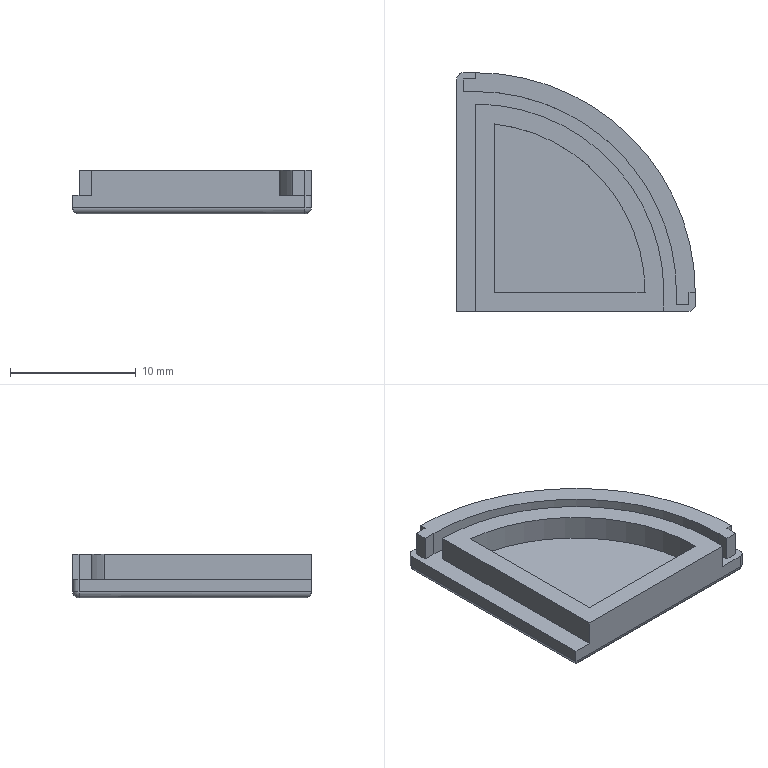Part | SolidWorks | features Extrusion 1, Fillet 1, ICE 1 | 1 solid | 34 faces | box 19 x 19 x 3.5 mm | volume 674.646 mm3 | plane 21 | cylinder 10 | sphere 2 | torus 1 | commonest cylinder face diameters 1 x6 27 x1 30 x1 32 x1 35 x1
STEP:
#1=CARTESIAN_POINT('',(16.5,0.,1.5));
#2=VERTEX_POINT('',#1);
#3=CARTESIAN_POINT('',(18.5,0.,1.5));
#4=VERTEX_POINT('',#3);
#5=CARTESIAN_POINT('',(19.,0.,1.5));
#6=DIRECTION('',(1.,0.,0.));
#7=VECTOR('',#6,1000.);
#8=LINE('',#5,#7);
#9=EDGE_CURVE('',#2,#4,#8,.T.);
#10=ORIENTED_EDGE('',*,*,#9,.T.);
#11=CARTESIAN_POINT('',(19.,0.5,1.5));
#12=VERTEX_POINT('',#11);
#13=CARTESIAN_POINT('',(18.5,0.5,1.5));
#14=DIRECTION('',(0.,0.,1.));
#15=DIRECTION('',(-1.,0.,0.));
#16=AXIS2_PLACEMENT_3D('',#13,#14,#15);
#17=CIRCLE('',#16,0.5);
#18=EDGE_CURVE('',#4,#12,#17,.T.);
#19=ORIENTED_EDGE('',*,*,#18,.T.);
#20=CARTESIAN_POINT('',(19.,1.5,1.5));
#21=VERTEX_POINT('',#20);
#22=CARTESIAN_POINT('',(19.,1.5,1.5));
#23=DIRECTION('',(0.,1.,0.));
#24=VECTOR('',#23,1000.);
#25=LINE('',#22,#24);
#26=EDGE_CURVE('',#12,#21,#25,.T.);
#27=ORIENTED_EDGE('',*,*,#26,.T.);
#28=CARTESIAN_POINT('',(18.5,1.5,1.5));
#29=VERTEX_POINT('',#28);
#30=CARTESIAN_POINT('',(18.5,1.5,1.5));
#31=DIRECTION('',(1.,0.,0.));
#32=VECTOR('',#31,1000.);
#33=LINE('',#30,#32);
#34=EDGE_CURVE('',#29,#21,#33,.T.);
#35=ORIENTED_EDGE('',*,*,#34,.F.);
#36=CARTESIAN_POINT('',(18.5,0.5,1.5));
#37=VERTEX_POINT('',#36);
#38=CARTESIAN_POINT('',(18.5,0.5,1.5));
#39=DIRECTION('',(0.,1.,0.));
#40=VECTOR('',#39,1000.);
#41=LINE('',#38,#40);
#42=EDGE_CURVE('',#37,#29,#41,.T.);
#43=ORIENTED_EDGE('',*,*,#42,.F.);
#44=CARTESIAN_POINT('',(17.5,0.5,1.5));
#45=VERTEX_POINT('',#44);
#46=CARTESIAN_POINT('',(17.5,0.5,1.5));
#47=DIRECTION('',(1.,0.,0.));
#48=VECTOR('',#47,1000.);
#49=LINE('',#46,#48);
#50=EDGE_CURVE('',#45,#37,#49,.T.);
#51=ORIENTED_EDGE('',*,*,#50,.F.);
#52=CARTESIAN_POINT('',(17.5,1.5,1.5));
#53=VERTEX_POINT('',#52);
#54=CARTESIAN_POINT('',(17.5,1.5,1.5));
#55=DIRECTION('',(0.,-1.,0.));
#56=VECTOR('',#55,1000.);
#57=LINE('',#54,#56);
#58=EDGE_CURVE('',#53,#45,#57,.T.);
#59=ORIENTED_EDGE('',*,*,#58,.F.);
#60=CARTESIAN_POINT('',(1.5,17.5,1.5));
#61=VERTEX_POINT('',#60);
#62=CARTESIAN_POINT('',(1.5,1.5,1.5));
#63=DIRECTION('',(0.,0.,-1.));
#64=DIRECTION('',(-1.,0.,0.));
#65=AXIS2_PLACEMENT_3D('',#62,#63,#64);
#66=CIRCLE('',#65,16.);
#67=EDGE_CURVE('',#61,#53,#66,.T.);
#68=ORIENTED_EDGE('',*,*,#67,.F.);
#69=CARTESIAN_POINT('',(0.5,17.5,1.5));
#70=VERTEX_POINT('',#69);
#71=CARTESIAN_POINT('',(0.5,17.5,1.5));
#72=DIRECTION('',(1.,0.,0.));
#73=VECTOR('',#72,1000.);
#74=LINE('',#71,#73);
#75=EDGE_CURVE('',#70,#61,#74,.T.);
#76=ORIENTED_EDGE('',*,*,#75,.F.);
#77=CARTESIAN_POINT('',(0.5,18.5,1.5));
#78=VERTEX_POINT('',#77);
#79=CARTESIAN_POINT('',(0.5,18.5,1.5));
#80=DIRECTION('',(0.,-1.,0.));
#81=VECTOR('',#80,1000.);
#82=LINE('',#79,#81);
#83=EDGE_CURVE('',#78,#70,#82,.T.);
#84=ORIENTED_EDGE('',*,*,#83,.F.);
#85=CARTESIAN_POINT('',(1.5,18.5,1.5));
#86=VERTEX_POINT('',#85);
#87=CARTESIAN_POINT('',(1.5,18.5,1.5));
#88=DIRECTION('',(-1.,0.,0.));
#89=VECTOR('',#88,1000.);
#90=LINE('',#87,#89);
#91=EDGE_CURVE('',#86,#78,#90,.T.);
#92=ORIENTED_EDGE('',*,*,#91,.F.);
#93=CARTESIAN_POINT('',(1.5,19.,1.5));
#94=VERTEX_POINT('',#93);
#95=CARTESIAN_POINT('',(1.5,19.,1.5));
#96=DIRECTION('',(0.,-1.,0.));
#97=VECTOR('',#96,1000.);
#98=LINE('',#95,#97);
#99=EDGE_CURVE('',#94,#86,#98,.T.);
#100=ORIENTED_EDGE('',*,*,#99,.F.);
#101=CARTESIAN_POINT('',(0.5,19.,1.5));
#102=VERTEX_POINT('',#101);
#103=CARTESIAN_POINT('',(0.,19.,1.5));
#104=DIRECTION('',(-1.,0.,0.));
#105=VECTOR('',#104,1000.);
#106=LINE('',#103,#105);
#107=EDGE_CURVE('',#94,#102,#106,.T.);
#108=ORIENTED_EDGE('',*,*,#107,.T.);
#109=CARTESIAN_POINT('',(0.,18.5,1.5));
#110=VERTEX_POINT('',#109);
#111=CARTESIAN_POINT('',(0.5,18.5,1.5));
#112=DIRECTION('',(0.,0.,1.));
#113=DIRECTION('',(-1.,0.,0.));
#114=AXIS2_PLACEMENT_3D('',#111,#112,#113);
#115=CIRCLE('',#114,0.5);
#116=EDGE_CURVE('',#102,#110,#115,.T.);
#117=ORIENTED_EDGE('',*,*,#116,.T.);
#118=CARTESIAN_POINT('',(0.,0.,1.5));
#119=VERTEX_POINT('',#118);
#120=CARTESIAN_POINT('',(0.,0.,1.5));
#121=DIRECTION('',(0.,-1.,0.));
#122=VECTOR('',#121,1000.);
#123=LINE('',#120,#122);
#124=EDGE_CURVE('',#110,#119,#123,.T.);
#125=ORIENTED_EDGE('',*,*,#124,.T.);
#126=CARTESIAN_POINT('',(1.5,0.,1.5));
#127=VERTEX_POINT('',#126);
#128=CARTESIAN_POINT('',(19.,0.,1.5));
#129=DIRECTION('',(1.,0.,0.));
#130=VECTOR('',#129,1000.);
#131=LINE('',#128,#130);
#132=EDGE_CURVE('',#119,#127,#131,.T.);
#133=ORIENTED_EDGE('',*,*,#132,.T.);
#134=CARTESIAN_POINT('',(1.5,16.5,1.5));
#135=VERTEX_POINT('',#134);
#136=CARTESIAN_POINT('',(1.5,16.5,1.5));
#137=DIRECTION('',(0.,-1.,0.));
#138=VECTOR('',#137,1000.);
#139=LINE('',#136,#138);
#140=EDGE_CURVE('',#135,#127,#139,.T.);
#141=ORIENTED_EDGE('',*,*,#140,.F.);
#142=CARTESIAN_POINT('',(16.5,1.5,1.5));
#143=VERTEX_POINT('',#142);
#144=CARTESIAN_POINT('',(1.5,1.5,1.5));
#145=DIRECTION('',(0.,0.,1.));
#146=DIRECTION('',(1.,0.,0.));
#147=AXIS2_PLACEMENT_3D('',#144,#145,#146);
#148=CIRCLE('',#147,15.);
#149=EDGE_CURVE('',#143,#135,#148,.T.);
#150=ORIENTED_EDGE('',*,*,#149,.F.);
#151=CARTESIAN_POINT('',(16.5,0.,1.5));
#152=DIRECTION('',(0.,1.,0.));
#153=VECTOR('',#152,1000.);
#154=LINE('',#151,#153);
#155=EDGE_CURVE('',#2,#143,#154,.T.);
#156=ORIENTED_EDGE('',*,*,#155,.F.);
#157=EDGE_LOOP('',(#10,#19,#27,#35,#43,#51,#59,#68,#76,#84,#92,#100,#108,#117,#125,#133,#141,#150,#156));
#158=FACE_OUTER_BOUND('',#157,.T.);
#159=CARTESIAN_POINT('',(1.5,1.5,1.5));
#160=DIRECTION('',(0.,0.,-1.));
#161=DIRECTION('',(-1.,0.,0.));
#162=AXIS2_PLACEMENT_3D('',#159,#160,#161);
#163=PLANE('',#162);
#164=ADVANCED_FACE('',(#158),#163,.F.);
#165=CARTESIAN_POINT('',(0.,0.,0.5));
#166=VERTEX_POINT('',#165);
#167=CARTESIAN_POINT('',(18.5,0.,0.5));
#168=VERTEX_POINT('',#167);
#169=CARTESIAN_POINT('',(19.,0.,0.5));
#170=DIRECTION('',(1.,0.,0.));
#171=VECTOR('',#170,1000.);
#172=LINE('',#169,#171);
#173=EDGE_CURVE('',#166,#168,#172,.T.);
#174=ORIENTED_EDGE('',*,*,#173,.T.);
#175=CARTESIAN_POINT('',(18.5,0.,1.5));
#176=DIRECTION('',(0.,0.,1.));
#177=VECTOR('',#176,1000.);
#178=LINE('',#175,#177);
#179=EDGE_CURVE('',#168,#4,#178,.T.);
#180=ORIENTED_EDGE('',*,*,#179,.T.);
#181=ORIENTED_EDGE('',*,*,#9,.F.);
#182=CARTESIAN_POINT('',(16.5,0.,3.5));
#183=VERTEX_POINT('',#182);
#184=CARTESIAN_POINT('',(16.5,0.,3.5));
#185=DIRECTION('',(0.,0.,-1.));
#186=VECTOR('',#185,1000.);
#187=LINE('',#184,#186);
#188=EDGE_CURVE('',#183,#2,#187,.T.);
#189=ORIENTED_EDGE('',*,*,#188,.F.);
#190=CARTESIAN_POINT('',(1.5,0.,3.5));
#191=VERTEX_POINT('',#190);
#192=CARTESIAN_POINT('',(1.5,0.,3.5));
#193=DIRECTION('',(1.,0.,0.));
#194=VECTOR('',#193,1000.);
#195=LINE('',#192,#194);
#196=EDGE_CURVE('',#191,#183,#195,.T.);
#197=ORIENTED_EDGE('',*,*,#196,.F.);
#198=CARTESIAN_POINT('',(1.5,0.,3.5));
#199=DIRECTION('',(0.,0.,-1.));
#200=VECTOR('',#199,1000.);
#201=LINE('',#198,#200);
#202=EDGE_CURVE('',#191,#127,#201,.T.);
#203=ORIENTED_EDGE('',*,*,#202,.T.);
#204=ORIENTED_EDGE('',*,*,#132,.F.);
#205=CARTESIAN_POINT('',(0.,0.,1.5));
#206=DIRECTION('',(0.,0.,-1.));
#207=VECTOR('',#206,1000.);
#208=LINE('',#205,#207);
#209=EDGE_CURVE('',#119,#166,#208,.T.);
#210=ORIENTED_EDGE('',*,*,#209,.T.);
#211=EDGE_LOOP('',(#174,#180,#181,#189,#197,#203,#204,#210));
#212=FACE_OUTER_BOUND('',#211,.T.);
#213=CARTESIAN_POINT('',(19.,0.,1.5));
#214=DIRECTION('',(0.,1.,0.));
#215=DIRECTION('',(0.,0.,1.));
#216=AXIS2_PLACEMENT_3D('',#213,#214,#215);
#217=PLANE('',#216);
#218=ADVANCED_FACE('',(#212),#217,.F.);
#219=CARTESIAN_POINT('',(19.,0.5,0.5));
#220=VERTEX_POINT('',#219);
#221=CARTESIAN_POINT('',(19.,0.5,1.5));
#222=DIRECTION('',(0.,0.,-1.));
#223=VECTOR('',#222,1000.);
#224=LINE('',#221,#223);
#225=EDGE_CURVE('',#12,#220,#224,.T.);
#226=ORIENTED_EDGE('',*,*,#225,.T.);
#227=CARTESIAN_POINT('',(19.,1.5,0.5));
#228=VERTEX_POINT('',#227);
#229=CARTESIAN_POINT('',(19.,1.5,0.5));
#230=DIRECTION('',(0.,1.,0.));
#231=VECTOR('',#230,1000.);
#232=LINE('',#229,#231);
#233=EDGE_CURVE('',#220,#228,#232,.T.);
#234=ORIENTED_EDGE('',*,*,#233,.T.);
#235=CARTESIAN_POINT('',(19.,1.5,1.5));
#236=DIRECTION('',(0.,0.,-1.));
#237=VECTOR('',#236,1000.);
#238=LINE('',#235,#237);
#239=EDGE_CURVE('',#21,#228,#238,.T.);
#240=ORIENTED_EDGE('',*,*,#239,.F.);
#241=ORIENTED_EDGE('',*,*,#26,.F.);
#242=EDGE_LOOP('',(#226,#234,#240,#241));
#243=FACE_OUTER_BOUND('',#242,.T.);
#244=CARTESIAN_POINT('',(19.,1.5,1.5));
#245=DIRECTION('',(-1.,0.,0.));
#246=DIRECTION('',(0.,0.,1.));
#247=AXIS2_PLACEMENT_3D('',#244,#245,#246);
#248=PLANE('',#247);
#249=ADVANCED_FACE('',(#243),#248,.F.);
#250=ORIENTED_EDGE('',*,*,#239,.T.);
#251=CARTESIAN_POINT('',(1.5,19.,0.5));
#252=VERTEX_POINT('',#251);
#253=CARTESIAN_POINT('',(1.5,1.5,0.5));
#254=DIRECTION('',(0.,0.,1.));
#255=DIRECTION('',(-1.,0.,0.));
#256=AXIS2_PLACEMENT_3D('',#253,#254,#255);
#257=CIRCLE('',#256,17.5);
#258=EDGE_CURVE('',#228,#252,#257,.T.);
#259=ORIENTED_EDGE('',*,*,#258,.T.);
#260=CARTESIAN_POINT('',(1.5,19.,1.5));
#261=DIRECTION('',(0.,0.,-1.));
#262=VECTOR('',#261,1000.);
#263=LINE('',#260,#262);
#264=EDGE_CURVE('',#94,#252,#263,.T.);
#265=ORIENTED_EDGE('',*,*,#264,.F.);
#266=CARTESIAN_POINT('',(1.5,19.,3.5));
#267=VERTEX_POINT('',#266);
#268=CARTESIAN_POINT('',(1.5,19.,3.5));
#269=DIRECTION('',(0.,0.,-1.));
#270=VECTOR('',#269,1000.);
#271=LINE('',#268,#270);
#272=EDGE_CURVE('',#267,#94,#271,.T.);
#273=ORIENTED_EDGE('',*,*,#272,.F.);
#274=CARTESIAN_POINT('',(19.,1.5,3.5));
#275=VERTEX_POINT('',#274);
#276=CARTESIAN_POINT('',(1.5,1.5,3.5));
#277=DIRECTION('',(0.,0.,1.));
#278=DIRECTION('',(1.,0.,0.));
#279=AXIS2_PLACEMENT_3D('',#276,#277,#278);
#280=CIRCLE('',#279,17.5);
#281=EDGE_CURVE('',#275,#267,#280,.T.);
#282=ORIENTED_EDGE('',*,*,#281,.F.);
#283=CARTESIAN_POINT('',(19.,1.5,3.5));
#284=DIRECTION('',(0.,0.,-1.));
#285=VECTOR('',#284,1000.);
#286=LINE('',#283,#285);
#287=EDGE_CURVE('',#275,#21,#286,.T.);
#288=ORIENTED_EDGE('',*,*,#287,.T.);
#289=EDGE_LOOP('',(#250,#259,#265,#273,#282,#288));
#290=FACE_OUTER_BOUND('',#289,.T.);
#291=CARTESIAN_POINT('',(1.5,1.5,1.5));
#292=DIRECTION('',(0.,0.,-1.));
#293=DIRECTION('',(-1.,0.,0.));
#294=AXIS2_PLACEMENT_3D('',#291,#292,#293);
#295=CYLINDRICAL_SURFACE('',#294,17.5);
#296=ADVANCED_FACE('',(#290),#295,.T.);
#297=ORIENTED_EDGE('',*,*,#264,.T.);
#298=CARTESIAN_POINT('',(0.5,19.,0.5));
#299=VERTEX_POINT('',#298);
#300=CARTESIAN_POINT('',(0.,19.,0.5));
#301=DIRECTION('',(-1.,0.,0.));
#302=VECTOR('',#301,1000.);
#303=LINE('',#300,#302);
#304=EDGE_CURVE('',#252,#299,#303,.T.);
#305=ORIENTED_EDGE('',*,*,#304,.T.);
#306=CARTESIAN_POINT('',(0.5,19.,1.5));
#307=DIRECTION('',(0.,0.,1.));
#308=VECTOR('',#307,1000.);
#309=LINE('',#306,#308);
#310=EDGE_CURVE('',#299,#102,#309,.T.);
#311=ORIENTED_EDGE('',*,*,#310,.T.);
#312=ORIENTED_EDGE('',*,*,#107,.F.);
#313=EDGE_LOOP('',(#297,#305,#311,#312));
#314=FACE_OUTER_BOUND('',#313,.T.);
#315=CARTESIAN_POINT('',(0.,19.,1.5));
#316=DIRECTION('',(0.,-1.,0.));
#317=DIRECTION('',(0.,0.,-1.));
#318=AXIS2_PLACEMENT_3D('',#315,#316,#317);
#319=PLANE('',#318);
#320=ADVANCED_FACE('',(#314),#319,.F.);
#321=ORIENTED_EDGE('',*,*,#124,.F.);
#322=CARTESIAN_POINT('',(0.,18.5,0.5));
#323=VERTEX_POINT('',#322);
#324=CARTESIAN_POINT('',(0.,18.5,1.5));
#325=DIRECTION('',(0.,0.,-1.));
#326=VECTOR('',#325,1000.);
#327=LINE('',#324,#326);
#328=EDGE_CURVE('',#110,#323,#327,.T.);
#329=ORIENTED_EDGE('',*,*,#328,.T.);
#330=CARTESIAN_POINT('',(0.,0.,0.5));
#331=DIRECTION('',(0.,-1.,0.));
#332=VECTOR('',#331,1000.);
#333=LINE('',#330,#332);
#334=EDGE_CURVE('',#323,#166,#333,.T.);
#335=ORIENTED_EDGE('',*,*,#334,.T.);
#336=ORIENTED_EDGE('',*,*,#209,.F.);
#337=EDGE_LOOP('',(#321,#329,#335,#336));
#338=FACE_OUTER_BOUND('',#337,.T.);
#339=CARTESIAN_POINT('',(0.,0.,1.5));
#340=DIRECTION('',(1.,0.,0.));
#341=DIRECTION('',(0.,0.,-1.));
#342=AXIS2_PLACEMENT_3D('',#339,#340,#341);
#343=PLANE('',#342);
#344=ADVANCED_FACE('',(#338),#343,.F.);
#345=CARTESIAN_POINT('',(18.5,0.5,0.));
#346=VERTEX_POINT('',#345);
#347=CARTESIAN_POINT('',(0.5,0.5,0.));
#348=VERTEX_POINT('',#347);
#349=CARTESIAN_POINT('',(0.,0.5,0.));
#350=DIRECTION('',(-1.,0.,0.));
#351=VECTOR('',#350,1000.);
#352=LINE('',#349,#351);
#353=EDGE_CURVE('',#346,#348,#352,.T.);
#354=ORIENTED_EDGE('',*,*,#353,.T.);
#355=CARTESIAN_POINT('',(0.5,18.5,0.));
#356=VERTEX_POINT('',#355);
#357=CARTESIAN_POINT('',(0.5,19.,0.));
#358=DIRECTION('',(0.,1.,0.));
#359=VECTOR('',#358,1000.);
#360=LINE('',#357,#359);
#361=EDGE_CURVE('',#348,#356,#360,.T.);
#362=ORIENTED_EDGE('',*,*,#361,.T.);
#363=CARTESIAN_POINT('',(1.5,18.5,0.));
#364=VERTEX_POINT('',#363);
#365=CARTESIAN_POINT('',(1.5,18.5,0.));
#366=DIRECTION('',(1.,0.,0.));
#367=VECTOR('',#366,1000.);
#368=LINE('',#365,#367);
#369=EDGE_CURVE('',#356,#364,#368,.T.);
#370=ORIENTED_EDGE('',*,*,#369,.T.);
#371=CARTESIAN_POINT('',(18.5,1.5,0.));
#372=VERTEX_POINT('',#371);
#373=CARTESIAN_POINT('',(1.5,1.5,0.));
#374=DIRECTION('',(0.,0.,-1.));
#375=DIRECTION('',(-1.,0.,0.));
#376=AXIS2_PLACEMENT_3D('',#373,#374,#375);
#377=CIRCLE('',#376,17.);
#378=EDGE_CURVE('',#364,#372,#377,.T.);
#379=ORIENTED_EDGE('',*,*,#378,.T.);
#380=CARTESIAN_POINT('',(18.5,0.,0.));
#381=DIRECTION('',(0.,-1.,0.));
#382=VECTOR('',#381,1000.);
#383=LINE('',#380,#382);
#384=EDGE_CURVE('',#372,#346,#383,.T.);
#385=ORIENTED_EDGE('',*,*,#384,.T.);
#386=EDGE_LOOP('',(#354,#362,#370,#379,#385));
#387=FACE_OUTER_BOUND('',#386,.T.);
#388=CARTESIAN_POINT('',(1.5,1.5,0.));
#389=DIRECTION('',(0.,0.,-1.));
#390=DIRECTION('',(-1.,0.,0.));
#391=AXIS2_PLACEMENT_3D('',#388,#389,#390);
#392=PLANE('',#391);
#393=ADVANCED_FACE('',(#387),#392,.T.);
#394=ORIENTED_EDGE('',*,*,#99,.T.);
#395=CARTESIAN_POINT('',(1.5,18.5,3.5));
#396=VERTEX_POINT('',#395);
#397=CARTESIAN_POINT('',(1.5,18.5,3.5));
#398=DIRECTION('',(0.,0.,-1.));
#399=VECTOR('',#398,1000.);
#400=LINE('',#397,#399);
#401=EDGE_CURVE('',#396,#86,#400,.T.);
#402=ORIENTED_EDGE('',*,*,#401,.F.);
#403=CARTESIAN_POINT('',(1.5,19.,3.5));
#404=DIRECTION('',(0.,-1.,0.));
#405=VECTOR('',#404,1000.);
#406=LINE('',#403,#405);
#407=EDGE_CURVE('',#267,#396,#406,.T.);
#408=ORIENTED_EDGE('',*,*,#407,.F.);
#409=ORIENTED_EDGE('',*,*,#272,.T.);
#410=EDGE_LOOP('',(#394,#402,#408,#409));
#411=FACE_OUTER_BOUND('',#410,.T.);
#412=CARTESIAN_POINT('',(1.5,19.,3.5));
#413=DIRECTION('',(1.,0.,0.));
#414=DIRECTION('',(0.,0.,-1.));
#415=AXIS2_PLACEMENT_3D('',#412,#413,#414);
#416=PLANE('',#415);
#417=ADVANCED_FACE('',(#411),#416,.F.);
#418=ORIENTED_EDGE('',*,*,#91,.T.);
#419=CARTESIAN_POINT('',(0.5,18.5,3.5));
#420=VERTEX_POINT('',#419);
#421=CARTESIAN_POINT('',(0.5,18.5,3.5));
#422=DIRECTION('',(0.,0.,-1.));
#423=VECTOR('',#422,1000.);
#424=LINE('',#421,#423);
#425=EDGE_CURVE('',#420,#78,#424,.T.);
#426=ORIENTED_EDGE('',*,*,#425,.F.);
#427=CARTESIAN_POINT('',(1.5,18.5,3.5));
#428=DIRECTION('',(-1.,0.,0.));
#429=VECTOR('',#428,1000.);
#430=LINE('',#427,#429);
#431=EDGE_CURVE('',#396,#420,#430,.T.);
#432=ORIENTED_EDGE('',*,*,#431,.F.);
#433=ORIENTED_EDGE('',*,*,#401,.T.);
#434=EDGE_LOOP('',(#418,#426,#432,#433));
#435=FACE_OUTER_BOUND('',#434,.T.);
#436=CARTESIAN_POINT('',(1.5,18.5,3.5));
#437=DIRECTION('',(0.,-1.,0.));
#438=DIRECTION('',(0.,0.,-1.));
#439=AXIS2_PLACEMENT_3D('',#436,#437,#438);
#440=PLANE('',#439);
#441=ADVANCED_FACE('',(#435),#440,.F.);
#442=ORIENTED_EDGE('',*,*,#83,.T.);
#443=CARTESIAN_POINT('',(0.5,17.5,3.5));
#444=VERTEX_POINT('',#443);
#445=CARTESIAN_POINT('',(0.5,17.5,3.5));
#446=DIRECTION('',(0.,0.,-1.));
#447=VECTOR('',#446,1000.);
#448=LINE('',#445,#447);
#449=EDGE_CURVE('',#444,#70,#448,.T.);
#450=ORIENTED_EDGE('',*,*,#449,.F.);
#451=CARTESIAN_POINT('',(0.5,18.5,3.5));
#452=DIRECTION('',(0.,-1.,0.));
#453=VECTOR('',#452,1000.);
#454=LINE('',#451,#453);
#455=EDGE_CURVE('',#420,#444,#454,.T.);
#456=ORIENTED_EDGE('',*,*,#455,.F.);
#457=ORIENTED_EDGE('',*,*,#425,.T.);
#458=EDGE_LOOP('',(#442,#450,#456,#457));
#459=FACE_OUTER_BOUND('',#458,.T.);
#460=CARTESIAN_POINT('',(0.5,18.5,3.5));
#461=DIRECTION('',(1.,0.,0.));
#462=DIRECTION('',(0.,0.,-1.));
#463=AXIS2_PLACEMENT_3D('',#460,#461,#462);
#464=PLANE('',#463);
#465=ADVANCED_FACE('',(#459),#464,.F.);
#466=ORIENTED_EDGE('',*,*,#75,.T.);
#467=CARTESIAN_POINT('',(1.5,17.5,3.5));
#468=VERTEX_POINT('',#467);
#469=CARTESIAN_POINT('',(1.5,17.5,3.5));
#470=DIRECTION('',(0.,0.,-1.));
#471=VECTOR('',#470,1000.);
#472=LINE('',#469,#471);
#473=EDGE_CURVE('',#468,#61,#472,.T.);
#474=ORIENTED_EDGE('',*,*,#473,.F.);
#475=CARTESIAN_POINT('',(0.5,17.5,3.5));
#476=DIRECTION('',(1.,0.,0.));
#477=VECTOR('',#476,1000.);
#478=LINE('',#475,#477);
#479=EDGE_CURVE('',#444,#468,#478,.T.);
#480=ORIENTED_EDGE('',*,*,#479,.F.);
#481=ORIENTED_EDGE('',*,*,#449,.T.);
#482=EDGE_LOOP('',(#466,#474,#480,#481));
#483=FACE_OUTER_BOUND('',#482,.T.);
#484=CARTESIAN_POINT('',(0.5,17.5,3.5));
#485=DIRECTION('',(0.,1.,0.));
#486=DIRECTION('',(0.,0.,1.));
#487=AXIS2_PLACEMENT_3D('',#484,#485,#486);
#488=PLANE('',#487);
#489=ADVANCED_FACE('',(#483),#488,.F.);
#490=ORIENTED_EDGE('',*,*,#67,.T.);
#491=CARTESIAN_POINT('',(17.5,1.5,3.5));
#492=VERTEX_POINT('',#491);
#493=CARTESIAN_POINT('',(17.5,1.5,3.5));
#494=DIRECTION('',(0.,0.,-1.));
#495=VECTOR('',#494,1000.);
#496=LINE('',#493,#495);
#497=EDGE_CURVE('',#492,#53,#496,.T.);
#498=ORIENTED_EDGE('',*,*,#497,.F.);
#499=CARTESIAN_POINT('',(1.5,1.5,3.5));
#500=DIRECTION('',(0.,0.,-1.));
#501=DIRECTION('',(-1.,0.,0.));
#502=AXIS2_PLACEMENT_3D('',#499,#500,#501);
#503=CIRCLE('',#502,16.);
#504=EDGE_CURVE('',#468,#492,#503,.T.);
#505=ORIENTED_EDGE('',*,*,#504,.F.);
#506=ORIENTED_EDGE('',*,*,#473,.T.);
#507=EDGE_LOOP('',(#490,#498,#505,#506));
#508=FACE_OUTER_BOUND('',#507,.T.);
#509=CARTESIAN_POINT('',(1.5,1.5,3.5));
#510=DIRECTION('',(0.,0.,-1.));
#511=DIRECTION('',(-1.,0.,0.));
#512=AXIS2_PLACEMENT_3D('',#509,#510,#511);
#513=CYLINDRICAL_SURFACE('',#512,16.);
#514=ADVANCED_FACE('',(#508),#513,.F.);
#515=ORIENTED_EDGE('',*,*,#58,.T.);
#516=CARTESIAN_POINT('',(17.5,0.5,3.5));
#517=VERTEX_POINT('',#516);
#518=CARTESIAN_POINT('',(17.5,0.5,3.5));
#519=DIRECTION('',(0.,0.,-1.));
#520=VECTOR('',#519,1000.);
#521=LINE('',#518,#520);
#522=EDGE_CURVE('',#517,#45,#521,.T.);
#523=ORIENTED_EDGE('',*,*,#522,.F.);
#524=CARTESIAN_POINT('',(17.5,1.5,3.5));
#525=DIRECTION('',(0.,-1.,0.));
#526=VECTOR('',#525,1000.);
#527=LINE('',#524,#526);
#528=EDGE_CURVE('',#492,#517,#527,.T.);
#529=ORIENTED_EDGE('',*,*,#528,.F.);
#530=ORIENTED_EDGE('',*,*,#497,.T.);
#531=EDGE_LOOP('',(#515,#523,#529,#530));
#532=FACE_OUTER_BOUND('',#531,.T.);
#533=CARTESIAN_POINT('',(17.5,1.5,3.5));
#534=DIRECTION('',(1.,0.,0.));
#535=DIRECTION('',(0.,0.,-1.));
#536=AXIS2_PLACEMENT_3D('',#533,#534,#535);
#537=PLANE('',#536);
#538=ADVANCED_FACE('',(#532),#537,.F.);
#539=ORIENTED_EDGE('',*,*,#50,.T.);
#540=CARTESIAN_POINT('',(18.5,0.5,3.5));
#541=VERTEX_POINT('',#540);
#542=CARTESIAN_POINT('',(18.5,0.5,3.5));
#543=DIRECTION('',(0.,0.,-1.));
#544=VECTOR('',#543,1000.);
#545=LINE('',#542,#544);
#546=EDGE_CURVE('',#541,#37,#545,.T.);
#547=ORIENTED_EDGE('',*,*,#546,.F.);
#548=CARTESIAN_POINT('',(17.5,0.5,3.5));
#549=DIRECTION('',(1.,0.,0.));
#550=VECTOR('',#549,1000.);
#551=LINE('',#548,#550);
#552=EDGE_CURVE('',#517,#541,#551,.T.);
#553=ORIENTED_EDGE('',*,*,#552,.F.);
#554=ORIENTED_EDGE('',*,*,#522,.T.);
#555=EDGE_LOOP('',(#539,#547,#553,#554));
#556=FACE_OUTER_BOUND('',#555,.T.);
#557=CARTESIAN_POINT('',(17.5,0.5,3.5));
#558=DIRECTION('',(0.,1.,0.));
#559=DIRECTION('',(0.,0.,1.));
#560=AXIS2_PLACEMENT_3D('',#557,#558,#559);
#561=PLANE('',#560);
#562=ADVANCED_FACE('',(#556),#561,.F.);
#563=ORIENTED_EDGE('',*,*,#42,.T.);
#564=CARTESIAN_POINT('',(18.5,1.5,3.5));
#565=VERTEX_POINT('',#564);
#566=CARTESIAN_POINT('',(18.5,1.5,3.5));
#567=DIRECTION('',(0.,0.,-1.));
#568=VECTOR('',#567,1000.);
#569=LINE('',#566,#568);
#570=EDGE_CURVE('',#565,#29,#569,.T.);
#571=ORIENTED_EDGE('',*,*,#570,.F.);
#572=CARTESIAN_POINT('',(18.5,0.5,3.5));
#573=DIRECTION('',(0.,1.,0.));
#574=VECTOR('',#573,1000.);
#575=LINE('',#572,#574);
#576=EDGE_CURVE('',#541,#565,#575,.T.);
#577=ORIENTED_EDGE('',*,*,#576,.F.);
#578=ORIENTED_EDGE('',*,*,#546,.T.);
#579=EDGE_LOOP('',(#563,#571,#577,#578));
#580=FACE_OUTER_BOUND('',#579,.T.);
#581=CARTESIAN_POINT('',(18.5,0.5,3.5));
#582=DIRECTION('',(-1.,0.,0.));
#583=DIRECTION('',(0.,0.,1.));
#584=AXIS2_PLACEMENT_3D('',#581,#582,#583);
#585=PLANE('',#584);
#586=ADVANCED_FACE('',(#580),#585,.F.);
#587=ORIENTED_EDGE('',*,*,#34,.T.);
#588=ORIENTED_EDGE('',*,*,#287,.F.);
#589=CARTESIAN_POINT('',(18.5,1.5,3.5));
#590=DIRECTION('',(1.,0.,0.));
#591=VECTOR('',#590,1000.);
#592=LINE('',#589,#591);
#593=EDGE_CURVE('',#565,#275,#592,.T.);
#594=ORIENTED_EDGE('',*,*,#593,.F.);
#595=ORIENTED_EDGE('',*,*,#570,.T.);
#596=EDGE_LOOP('',(#587,#588,#594,#595));
#597=FACE_OUTER_BOUND('',#596,.T.);
#598=CARTESIAN_POINT('',(18.5,1.5,3.5));
#599=DIRECTION('',(0.,1.,0.));
#600=DIRECTION('',(-1.,0.,0.));
#601=AXIS2_PLACEMENT_3D('',#598,#599,#600);
#602=PLANE('',#601);
#603=ADVANCED_FACE('',(#597),#602,.F.);
#604=ORIENTED_EDGE('',*,*,#281,.T.);
#605=ORIENTED_EDGE('',*,*,#407,.T.);
#606=ORIENTED_EDGE('',*,*,#431,.T.);
#607=ORIENTED_EDGE('',*,*,#455,.T.);
#608=ORIENTED_EDGE('',*,*,#479,.T.);
#609=ORIENTED_EDGE('',*,*,#504,.T.);
#610=ORIENTED_EDGE('',*,*,#528,.T.);
#611=ORIENTED_EDGE('',*,*,#552,.T.);
#612=ORIENTED_EDGE('',*,*,#576,.T.);
#613=ORIENTED_EDGE('',*,*,#593,.T.);
#614=EDGE_LOOP('',(#604,#605,#606,#607,#608,#609,#610,#611,#612,#613));
#615=FACE_OUTER_BOUND('',#614,.T.);
#616=CARTESIAN_POINT('',(1.5,1.5,3.5));
#617=DIRECTION('',(0.,0.,1.));
#618=DIRECTION('',(1.,0.,0.));
#619=AXIS2_PLACEMENT_3D('',#616,#617,#618);
#620=PLANE('',#619);
#621=ADVANCED_FACE('',(#615),#620,.T.);
#622=CARTESIAN_POINT('',(16.5,1.5,3.5));
#623=VERTEX_POINT('',#622);
#624=CARTESIAN_POINT('',(1.5,16.5,3.5));
#625=VERTEX_POINT('',#624);
#626=CARTESIAN_POINT('',(1.5,1.5,3.5));
#627=DIRECTION('',(0.,0.,1.));
#628=DIRECTION('',(1.,0.,0.));
#629=AXIS2_PLACEMENT_3D('',#626,#627,#628);
#630=CIRCLE('',#629,15.);
#631=EDGE_CURVE('',#623,#625,#630,.T.);
#632=ORIENTED_EDGE('',*,*,#631,.T.);
#633=CARTESIAN_POINT('',(1.5,16.5,3.5));
#634=DIRECTION('',(0.,-1.,0.));
#635=VECTOR('',#634,1000.);
#636=LINE('',#633,#635);
#637=EDGE_CURVE('',#625,#191,#636,.T.);
#638=ORIENTED_EDGE('',*,*,#637,.T.);
#639=ORIENTED_EDGE('',*,*,#196,.T.);
#640=CARTESIAN_POINT('',(16.5,0.,3.5));
#641=DIRECTION('',(0.,1.,0.));
#642=VECTOR('',#641,1000.);
#643=LINE('',#640,#642);
#644=EDGE_CURVE('',#183,#623,#643,.T.);
#645=ORIENTED_EDGE('',*,*,#644,.T.);
#646=EDGE_LOOP('',(#632,#638,#639,#645));
#647=FACE_OUTER_BOUND('',#646,.T.);
#648=CARTESIAN_POINT('',(3.,14.916,3.5));
#649=VERTEX_POINT('',#648);
#650=CARTESIAN_POINT('',(3.,1.5,3.5));
#651=VERTEX_POINT('',#650);
#652=CARTESIAN_POINT('',(3.,14.916,3.5));
#653=DIRECTION('',(0.,-1.,0.));
#654=VECTOR('',#653,1000.);
#655=LINE('',#652,#654);
#656=EDGE_CURVE('',#649,#651,#655,.T.);
#657=ORIENTED_EDGE('',*,*,#656,.F.);
#658=CARTESIAN_POINT('',(15.,1.5,3.5));
#659=VERTEX_POINT('',#658);
#660=CARTESIAN_POINT('',(1.5,1.5,3.5));
#661=DIRECTION('',(0.,0.,1.));
#662=DIRECTION('',(1.,0.,0.));
#663=AXIS2_PLACEMENT_3D('',#660,#661,#662);
#664=CIRCLE('',#663,13.5);
#665=EDGE_CURVE('',#659,#649,#664,.T.);
#666=ORIENTED_EDGE('',*,*,#665,.F.);
#667=CARTESIAN_POINT('',(3.,1.5,3.5));
#668=DIRECTION('',(1.,0.,0.));
#669=VECTOR('',#668,1000.);
#670=LINE('',#667,#669);
#671=EDGE_CURVE('',#651,#659,#670,.T.);
#672=ORIENTED_EDGE('',*,*,#671,.F.);
#673=EDGE_LOOP('',(#657,#666,#672));
#674=FACE_BOUND('',#673,.T.);
#675=CARTESIAN_POINT('',(1.5,1.5,3.5));
#676=DIRECTION('',(0.,0.,1.));
#677=DIRECTION('',(1.,0.,0.));
#678=AXIS2_PLACEMENT_3D('',#675,#676,#677);
#679=PLANE('',#678);
#680=ADVANCED_FACE('',(#647,#674),#679,.T.);
#681=ORIENTED_EDGE('',*,*,#149,.T.);
#682=CARTESIAN_POINT('',(1.5,16.5,3.5));
#683=DIRECTION('',(0.,0.,-1.));
#684=VECTOR('',#683,1000.);
#685=LINE('',#682,#684);
#686=EDGE_CURVE('',#625,#135,#685,.T.);
#687=ORIENTED_EDGE('',*,*,#686,.F.);
#688=ORIENTED_EDGE('',*,*,#631,.F.);
#689=CARTESIAN_POINT('',(16.5,1.5,3.5));
#690=DIRECTION('',(0.,0.,-1.));
#691=VECTOR('',#690,1000.);
#692=LINE('',#689,#691);
#693=EDGE_CURVE('',#623,#143,#692,.T.);
#694=ORIENTED_EDGE('',*,*,#693,.T.);
#695=EDGE_LOOP('',(#681,#687,#688,#694));
#696=FACE_OUTER_BOUND('',#695,.T.);
#697=CARTESIAN_POINT('',(1.5,1.5,3.5));
#698=DIRECTION('',(0.,0.,-1.));
#699=DIRECTION('',(-1.,0.,0.));
#700=AXIS2_PLACEMENT_3D('',#697,#698,#699);
#701=CYLINDRICAL_SURFACE('',#700,15.);
#702=ADVANCED_FACE('',(#696),#701,.T.);
#703=ORIENTED_EDGE('',*,*,#140,.T.);
#704=ORIENTED_EDGE('',*,*,#202,.F.);
#705=ORIENTED_EDGE('',*,*,#637,.F.);
#706=ORIENTED_EDGE('',*,*,#686,.T.);
#707=EDGE_LOOP('',(#703,#704,#705,#706));
#708=FACE_OUTER_BOUND('',#707,.T.);
#709=CARTESIAN_POINT('',(1.5,16.5,3.5));
#710=DIRECTION('',(1.,0.,0.));
#711=DIRECTION('',(0.,1.,0.));
#712=AXIS2_PLACEMENT_3D('',#709,#710,#711);
#713=PLANE('',#712);
#714=ADVANCED_FACE('',(#708),#713,.F.);
#715=ORIENTED_EDGE('',*,*,#155,.T.);
#716=ORIENTED_EDGE('',*,*,#693,.F.);
#717=ORIENTED_EDGE('',*,*,#644,.F.);
#718=ORIENTED_EDGE('',*,*,#188,.T.);
#719=EDGE_LOOP('',(#715,#716,#717,#718));
#720=FACE_OUTER_BOUND('',#719,.T.);
#721=CARTESIAN_POINT('',(16.5,0.,3.5));
#722=DIRECTION('',(-1.,0.,0.));
#723=DIRECTION('',(0.,0.,1.));
#724=AXIS2_PLACEMENT_3D('',#721,#722,#723);
#725=PLANE('',#724);
#726=ADVANCED_FACE('',(#720),#725,.F.);
#727=CARTESIAN_POINT('',(15.,1.5,1.5));
#728=VERTEX_POINT('',#727);
#729=CARTESIAN_POINT('',(3.,14.916,1.5));
#730=VERTEX_POINT('',#729);
#731=CARTESIAN_POINT('',(1.5,1.5,1.5));
#732=DIRECTION('',(0.,0.,1.));
#733=DIRECTION('',(1.,0.,0.));
#734=AXIS2_PLACEMENT_3D('',#731,#732,#733);
#735=CIRCLE('',#734,13.5);
#736=EDGE_CURVE('',#728,#730,#735,.T.);
#737=ORIENTED_EDGE('',*,*,#736,.F.);
#738=CARTESIAN_POINT('',(15.,1.5,3.5));
#739=DIRECTION('',(0.,0.,-1.));
#740=VECTOR('',#739,1000.);
#741=LINE('',#738,#740);
#742=EDGE_CURVE('',#659,#728,#741,.T.);
#743=ORIENTED_EDGE('',*,*,#742,.F.);
#744=ORIENTED_EDGE('',*,*,#665,.T.);
#745=CARTESIAN_POINT('',(3.,14.916,3.5));
#746=DIRECTION('',(0.,0.,-1.));
#747=VECTOR('',#746,1000.);
#748=LINE('',#745,#747);
#749=EDGE_CURVE('',#649,#730,#748,.T.);
#750=ORIENTED_EDGE('',*,*,#749,.T.);
#751=EDGE_LOOP('',(#737,#743,#744,#750));
#752=FACE_OUTER_BOUND('',#751,.T.);
#753=CARTESIAN_POINT('',(1.5,1.5,3.5));
#754=DIRECTION('',(0.,0.,-1.));
#755=DIRECTION('',(-1.,0.,0.));
#756=AXIS2_PLACEMENT_3D('',#753,#754,#755);
#757=CYLINDRICAL_SURFACE('',#756,13.5);
#758=ADVANCED_FACE('',(#752),#757,.F.);
#759=CARTESIAN_POINT('',(3.,1.5,1.5));
#760=VERTEX_POINT('',#759);
#761=CARTESIAN_POINT('',(3.,14.916,1.5));
#762=DIRECTION('',(0.,-1.,0.));
#763=VECTOR('',#762,1000.);
#764=LINE('',#761,#763);
#765=EDGE_CURVE('',#730,#760,#764,.T.);
#766=ORIENTED_EDGE('',*,*,#765,.F.);
#767=ORIENTED_EDGE('',*,*,#749,.F.);
#768=ORIENTED_EDGE('',*,*,#656,.T.);
#769=CARTESIAN_POINT('',(3.,1.5,3.5));
#770=DIRECTION('',(0.,0.,-1.));
#771=VECTOR('',#770,1000.);
#772=LINE('',#769,#771);
#773=EDGE_CURVE('',#651,#760,#772,.T.);
#774=ORIENTED_EDGE('',*,*,#773,.T.);
#775=EDGE_LOOP('',(#766,#767,#768,#774));
#776=FACE_OUTER_BOUND('',#775,.T.);
#777=CARTESIAN_POINT('',(3.,14.916,3.5));
#778=DIRECTION('',(1.,0.,0.));
#779=DIRECTION('',(0.,0.,-1.));
#780=AXIS2_PLACEMENT_3D('',#777,#778,#779);
#781=PLANE('',#780);
#782=ADVANCED_FACE('',(#776),#781,.T.);
#783=CARTESIAN_POINT('',(3.,1.5,1.5));
#784=DIRECTION('',(1.,0.,0.));
#785=VECTOR('',#784,1000.);
#786=LINE('',#783,#785);
#787=EDGE_CURVE('',#760,#728,#786,.T.);
#788=ORIENTED_EDGE('',*,*,#787,.F.);
#789=ORIENTED_EDGE('',*,*,#773,.F.);
#790=ORIENTED_EDGE('',*,*,#671,.T.);
#791=ORIENTED_EDGE('',*,*,#742,.T.);
#792=EDGE_LOOP('',(#788,#789,#790,#791));
#793=FACE_OUTER_BOUND('',#792,.T.);
#794=CARTESIAN_POINT('',(3.,1.5,3.5));
#795=DIRECTION('',(0.,1.,0.));
#796=DIRECTION('',(0.,0.,1.));
#797=AXIS2_PLACEMENT_3D('',#794,#795,#796);
#798=PLANE('',#797);
#799=ADVANCED_FACE('',(#793),#798,.T.);
#800=ORIENTED_EDGE('',*,*,#787,.T.);
#801=ORIENTED_EDGE('',*,*,#736,.T.);
#802=ORIENTED_EDGE('',*,*,#765,.T.);
#803=EDGE_LOOP('',(#800,#801,#802));
#804=FACE_OUTER_BOUND('',#803,.T.);
#805=CARTESIAN_POINT('',(1.5,1.5,1.5));
#806=DIRECTION('',(0.,0.,-1.));
#807=DIRECTION('',(-1.,0.,0.));
#808=AXIS2_PLACEMENT_3D('',#805,#806,#807);
#809=PLANE('',#808);
#810=ADVANCED_FACE('',(#804),#809,.F.);
#811=ORIENTED_EDGE('',*,*,#116,.F.);
#812=ORIENTED_EDGE('',*,*,#310,.F.);
#813=CARTESIAN_POINT('',(0.5,18.5,0.5));
#814=DIRECTION('',(0.,0.,-1.));
#815=DIRECTION('',(-1.,0.,0.));
#816=AXIS2_PLACEMENT_3D('',#813,#814,#815);
#817=CIRCLE('',#816,0.5);
#818=EDGE_CURVE('',#323,#299,#817,.T.);
#819=ORIENTED_EDGE('',*,*,#818,.F.);
#820=ORIENTED_EDGE('',*,*,#328,.F.);
#821=EDGE_LOOP('',(#811,#812,#819,#820));
#822=FACE_OUTER_BOUND('',#821,.T.);
#823=CARTESIAN_POINT('',(0.5,18.5,1.5));
#824=DIRECTION('',(0.,0.,-1.));
#825=DIRECTION('',(-1.,0.,0.));
#826=AXIS2_PLACEMENT_3D('',#823,#824,#825);
#827=CYLINDRICAL_SURFACE('',#826,0.5);
#828=ADVANCED_FACE('',(#822),#827,.T.);
#829=CARTESIAN_POINT('',(0.,0.,0.5));
#830=CARTESIAN_POINT('',(0.,0.,0.2071));
#831=CARTESIAN_POINT('',(0.2071,0.2071,0.));
#832=CARTESIAN_POINT('',(0.5,0.5,0.));
#833=(BOUNDED_CURVE()B_SPLINE_CURVE(3,(#829,#830,#831,#832),.UNSPECIFIED.,.F.,.F.)B_SPLINE_CURVE_WITH_KNOTS((4,4),(0.,1.571),.UNSPECIFIED.)CURVE()GEOMETRIC_REPRESENTATION_ITEM()RATIONAL_B_SPLINE_CURVE((1.,0.8047,0.8047,1.))REPRESENTATION_ITEM(''));
#834=EDGE_CURVE('',#166,#348,#833,.T.);
#835=ORIENTED_EDGE('',*,*,#834,.F.);
#836=ORIENTED_EDGE('',*,*,#334,.F.);
#837=CARTESIAN_POINT('',(0.5,18.5,0.5));
#838=DIRECTION('',(0.,1.,0.));
#839=DIRECTION('',(0.,0.,1.));
#840=AXIS2_PLACEMENT_3D('',#837,#838,#839);
#841=CIRCLE('',#840,0.5);
#842=EDGE_CURVE('',#356,#323,#841,.T.);
#843=ORIENTED_EDGE('',*,*,#842,.F.);
#844=ORIENTED_EDGE('',*,*,#361,.F.);
#845=EDGE_LOOP('',(#835,#836,#843,#844));
#846=FACE_OUTER_BOUND('',#845,.T.);
#847=CARTESIAN_POINT('',(0.5,0.,0.5));
#848=DIRECTION('',(0.,1.,0.));
#849=DIRECTION('',(0.,0.,1.));
#850=AXIS2_PLACEMENT_3D('',#847,#848,#849);
#851=CYLINDRICAL_SURFACE('',#850,0.5);
#852=ADVANCED_FACE('',(#846),#851,.T.);
#853=ORIENTED_EDGE('',*,*,#842,.T.);
#854=ORIENTED_EDGE('',*,*,#818,.T.);
#855=CARTESIAN_POINT('',(0.5,18.5,0.5));
#856=DIRECTION('',(1.,0.,0.));
#857=DIRECTION('',(0.,0.,1.));
#858=AXIS2_PLACEMENT_3D('',#855,#856,#857);
#859=CIRCLE('',#858,0.5);
#860=EDGE_CURVE('',#356,#299,#859,.T.);
#861=ORIENTED_EDGE('',*,*,#860,.F.);
#862=EDGE_LOOP('',(#853,#854,#861));
#863=FACE_OUTER_BOUND('',#862,.T.);
#864=CARTESIAN_POINT('',(0.5,18.5,0.5));
#865=DIRECTION('',(0.,1.,0.));
#866=DIRECTION('',(1.,0.,0.));
#867=AXIS2_PLACEMENT_3D('',#864,#865,#866);
#868=SPHERICAL_SURFACE('',#867,0.5);
#869=ADVANCED_FACE('',(#863),#868,.T.);
#870=ORIENTED_EDGE('',*,*,#834,.T.);
#871=ORIENTED_EDGE('',*,*,#353,.F.);
#872=CARTESIAN_POINT('',(18.5,0.5,0.5));
#873=DIRECTION('',(1.,0.,0.));
#874=DIRECTION('',(0.,0.,-1.));
#875=AXIS2_PLACEMENT_3D('',#872,#873,#874);
#876=CIRCLE('',#875,0.5);
#877=EDGE_CURVE('',#168,#346,#876,.T.);
#878=ORIENTED_EDGE('',*,*,#877,.F.);
#879=ORIENTED_EDGE('',*,*,#173,.F.);
#880=EDGE_LOOP('',(#870,#871,#878,#879));
#881=FACE_OUTER_BOUND('',#880,.T.);
#882=CARTESIAN_POINT('',(19.,0.5,0.5));
#883=DIRECTION('',(-1.,0.,0.));
#884=DIRECTION('',(0.,0.,1.));
#885=AXIS2_PLACEMENT_3D('',#882,#883,#884);
#886=CYLINDRICAL_SURFACE('',#885,0.5);
#887=ADVANCED_FACE('',(#881),#886,.T.);
#888=ORIENTED_EDGE('',*,*,#18,.F.);
#889=ORIENTED_EDGE('',*,*,#179,.F.);
#890=CARTESIAN_POINT('',(18.5,0.5,0.5));
#891=DIRECTION('',(0.,0.,-1.));
#892=DIRECTION('',(-1.,0.,0.));
#893=AXIS2_PLACEMENT_3D('',#890,#891,#892);
#894=CIRCLE('',#893,0.5);
#895=EDGE_CURVE('',#220,#168,#894,.T.);
#896=ORIENTED_EDGE('',*,*,#895,.F.);
#897=ORIENTED_EDGE('',*,*,#225,.F.);
#898=EDGE_LOOP('',(#888,#889,#896,#897));
#899=FACE_OUTER_BOUND('',#898,.T.);
#900=CARTESIAN_POINT('',(18.5,0.5,1.5));
#901=DIRECTION('',(0.,0.,-1.));
#902=DIRECTION('',(-1.,0.,0.));
#903=AXIS2_PLACEMENT_3D('',#900,#901,#902);
#904=CYLINDRICAL_SURFACE('',#903,0.5);
#905=ADVANCED_FACE('',(#899),#904,.T.);
#906=ORIENTED_EDGE('',*,*,#860,.T.);
#907=ORIENTED_EDGE('',*,*,#304,.F.);
#908=CARTESIAN_POINT('',(1.5,18.5,0.5));
#909=DIRECTION('',(1.,0.,0.));
#910=DIRECTION('',(0.,0.,-1.));
#911=AXIS2_PLACEMENT_3D('',#908,#909,#910);
#912=CIRCLE('',#911,0.5);
#913=EDGE_CURVE('',#364,#252,#912,.T.);
#914=ORIENTED_EDGE('',*,*,#913,.F.);
#915=ORIENTED_EDGE('',*,*,#369,.F.);
#916=EDGE_LOOP('',(#906,#907,#914,#915));
#917=FACE_OUTER_BOUND('',#916,.T.);
#918=CARTESIAN_POINT('',(0.,18.5,0.5));
#919=DIRECTION('',(1.,0.,0.));
#920=DIRECTION('',(0.,0.,-1.));
#921=AXIS2_PLACEMENT_3D('',#918,#919,#920);
#922=CYLINDRICAL_SURFACE('',#921,0.5);
#923=ADVANCED_FACE('',(#917),#922,.T.);
#924=ORIENTED_EDGE('',*,*,#895,.T.);
#925=ORIENTED_EDGE('',*,*,#877,.T.);
#926=CARTESIAN_POINT('',(18.5,0.5,0.5));
#927=DIRECTION('',(0.,1.,0.));
#928=DIRECTION('',(0.,0.,-1.));
#929=AXIS2_PLACEMENT_3D('',#926,#927,#928);
#930=CIRCLE('',#929,0.5);
#931=EDGE_CURVE('',#220,#346,#930,.T.);
#932=ORIENTED_EDGE('',*,*,#931,.F.);
#933=EDGE_LOOP('',(#924,#925,#932));
#934=FACE_OUTER_BOUND('',#933,.T.);
#935=CARTESIAN_POINT('',(18.5,0.5,0.5));
#936=DIRECTION('',(0.,1.,0.));
#937=DIRECTION('',(1.,0.,0.));
#938=AXIS2_PLACEMENT_3D('',#935,#936,#937);
#939=SPHERICAL_SURFACE('',#938,0.5);
#940=ADVANCED_FACE('',(#934),#939,.T.);
#941=ORIENTED_EDGE('',*,*,#913,.T.);
#942=ORIENTED_EDGE('',*,*,#258,.F.);
#943=CARTESIAN_POINT('',(18.5,1.5,0.5));
#944=DIRECTION('',(0.,-1.,0.));
#945=DIRECTION('',(0.,0.,-1.));
#946=AXIS2_PLACEMENT_3D('',#943,#944,#945);
#947=CIRCLE('',#946,0.5);
#948=EDGE_CURVE('',#372,#228,#947,.T.);
#949=ORIENTED_EDGE('',*,*,#948,.F.);
#950=ORIENTED_EDGE('',*,*,#378,.F.);
#951=EDGE_LOOP('',(#941,#942,#949,#950));
#952=FACE_OUTER_BOUND('',#951,.T.);
#953=CARTESIAN_POINT('',(1.5,1.5,0.5));
#954=DIRECTION('',(0.,0.,-1.));
#955=DIRECTION('',(-1.,0.,0.));
#956=AXIS2_PLACEMENT_3D('',#953,#954,#955);
#957=TOROIDAL_SURFACE('',#956,17.,0.5);
#958=ADVANCED_FACE('',(#952),#957,.T.);
#959=ORIENTED_EDGE('',*,*,#931,.T.);
#960=ORIENTED_EDGE('',*,*,#384,.F.);
#961=ORIENTED_EDGE('',*,*,#948,.T.);
#962=ORIENTED_EDGE('',*,*,#233,.F.);
#963=EDGE_LOOP('',(#959,#960,#961,#962));
#964=FACE_OUTER_BOUND('',#963,.T.);
#965=CARTESIAN_POINT('',(18.5,1.5,0.5));
#966=DIRECTION('',(0.,-1.,0.));
#967=DIRECTION('',(0.,0.,-1.));
#968=AXIS2_PLACEMENT_3D('',#965,#966,#967);
#969=CYLINDRICAL_SURFACE('',#968,0.5);
#970=ADVANCED_FACE('',(#964),#969,.T.);
#971=CLOSED_SHELL('',(#164,#218,#249,#296,#320,#344,#393,#417,#441,#465,#489,#514,#538,#562,#586,#603,#621,#680,#702,#714,#726,#758,#782,#799,#810,#828,#852,#869,#887,#905,#923,#940,#958,#970));
#972=MANIFOLD_SOLID_BREP('',#971);
#973=CARTESIAN_POINT('',(0.,0.,0.));
#974=DIRECTION('',(0.,0.,1.));
#975=DIRECTION('',(1.,0.,0.));
#976=AXIS2_PLACEMENT_3D('',#973,#974,#975);
#977=(LENGTH_UNIT()NAMED_UNIT(*)SI_UNIT(.MILLI.,.METRE.));
#978=UNCERTAINTY_MEASURE_WITH_UNIT(LENGTH_MEASURE(0.00001),#977,'','');
#979=(NAMED_UNIT(*)PLANE_ANGLE_UNIT()SI_UNIT($,.RADIAN.));
#980=(NAMED_UNIT(*)SI_UNIT($,.STERADIAN.)SOLID_ANGLE_UNIT());
#981=(GEOMETRIC_REPRESENTATION_CONTEXT(3)GLOBAL_UNCERTAINTY_ASSIGNED_CONTEXT((#978))GLOBAL_UNIT_ASSIGNED_CONTEXT((#977,#979,#980))REPRESENTATION_CONTEXT('',''));
#982=ADVANCED_BREP_SHAPE_REPRESENTATION('',(#972,#976),#981);